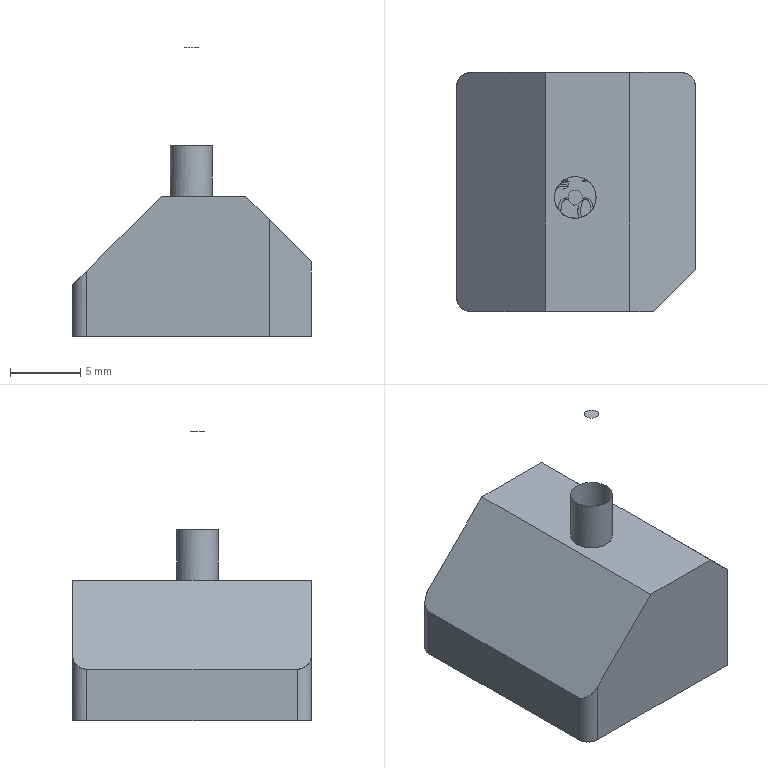NC program | PowerMill | posted with a generic post | part box 17 x 17 x 20.603 mm
Lines 37760 to 38492 of 42778:
N37857 M6
N37858 S18000 M03
N37859 G00 G90 X0.002 Y0.0
N37860 G43 Z9.803 H7
N37861
N37862 G05 P10000 R8
N37863 X9.8295 Y-5.6395
N37864 Z-14.7717
N37865 G01 Z-15.9717 F1200.0
N37866 X8.5944 Y-6.8746 Z-14.7367 F2000.0
N37867 X7.7228 Y-7.7462 Z-13.865
N37868 X7.4418 Y-8.0272 Z-13.5851
N37869 X7.1609 Y-8.3081 Z-13.3053
N37870 X6.8798 Y-8.5892 Z-13.0257
N37871 X6.7816 Y-8.6026 Z-12.9282
N37872 X7.0752 Y-8.309 Z-13.218
N37873 X7.8104 Y-7.5737 Z-13.9517
N37874 X8.6699 Y-6.7142 Z-14.8116
N37875 X9.8829 Y-5.5013 Z-16.025
N37876 X9.9345 Y-5.3648 Z-16.0781
N37877 X9.9048 Y-5.3945 Z-16.0479
N37878 X9.6356 Y-5.6637 Z-15.7768
N37879 X9.3656 Y-5.9337 Z-15.5072
N37880 X9.0957 Y-6.2036 Z-15.2376
N37881 X8.5216 Y-6.7777 Z-14.6631
N37882 X7.7273 Y-7.572 Z-13.8684
N37883 X7.3416 Y-7.9577 Z-13.4833
N37884 X6.9702 Y-8.3291 Z-13.112
N37885 X6.701 Y-8.5983 Z-12.8472
N37886 X6.6093 Y-8.6052 Z-12.756
N37887 X6.9039 Y-8.3106 Z-13.0467
N37888 X7.4978 Y-7.7166 Z-13.6392
N37889 X8.2992 Y-6.9152 Z-14.441
N37890 X9.0123 Y-6.2022 Z-15.1535
N37891 X9.3516 Y-5.8629 Z-15.4929
N37892 X9.6193 Y-5.5952 Z-15.7625
N37893 X9.9412 Y-5.2733 Z-16.0867
N37894 X9.9641 Y-5.2504 Z-16.1098
N37895 X9.9915 Y-5.1381 Z-16.1391
N37896 X9.872 Y-5.2576 Z-16.0174
N37897 X9.6054 Y-5.5242 Z-15.7477
N37898 X9.3296 Y-5.8 Z-15.4712
N37899 X8.9941 Y-6.1355 Z-15.1351
N37900 X8.2311 Y-6.8985 Z-14.3728
N37901 X7.4921 Y-7.6375 Z-13.6332
N37902 X7.1025 Y-8.0271 Z-13.2441
N37903 X6.782 Y-8.3476 Z-12.9248
N37904 X6.5202 Y-8.6094 Z-12.667
N37905 X6.4344 Y-8.6104 Z-12.5815
N37906 X6.6167 Y-8.428 Z-12.7612
N37907 X6.7988 Y-8.246 Z-12.9414
N37908 X6.9807 Y-8.0641 Z-13.1221
N37909 X7.3183 Y-7.7265 Z-13.4599
N37910 X7.9832 Y-7.0616 Z-14.1246
N37911 X8.8697 Y-6.1751 Z-15.0108
N37912 X9.2937 Y-5.751 Z-15.4354
N37913 X9.6371 Y-5.4076 Z-15.7792
N37914 X9.9348 Y-5.1099 Z-16.0802
N37915 X9.9922 Y-5.0526 Z-16.1388
N37916 X9.9871 Y-4.9728 Z-16.1343
N37917 X9.9382 Y-5.0217 Z-16.0844
N37918 X9.6271 Y-5.3328 Z-15.7697
N37919 X9.3152 Y-5.6447 Z-15.4566
N37920 X8.8493 Y-6.1106 Z-14.9908
N37921 X7.9104 Y-7.0495 Z-14.0519
N37922 X7.2311 Y-7.7288 Z-13.3727
N37923 X6.8845 Y-8.0754 Z-13.026
N37924 X6.7064 Y-8.2535 Z-12.8491
N37925 X6.528 Y-8.4319 Z-12.6726
N37926 X6.3494 Y-8.6105 Z-12.4966
N37927 X6.2647 Y-8.6104 Z-12.4118
N37928 X6.4471 Y-8.4279 Z-12.5916
N37929 X6.6293 Y-8.2457 Z-12.7719
N37930 X6.8113 Y-8.0638 Z-12.9527
N37931 X7.1489 Y-7.7261 Z-13.2905
N37932 X7.7898 Y-7.0853 Z-13.9313
N37933 X8.6032 Y-6.2719 Z-14.7447
N37934 X9.004 Y-5.871 Z-15.1458
N37935 X9.3524 Y-5.5226 Z-15.4932
N37936 X9.5245 Y-5.3505 Z-15.6664
N37937 X9.6998 Y-5.1753 Z-15.8414
N37938 X9.8121 Y-5.063 Z-15.9536
N37939 X9.9233 Y-4.9517 Z-16.0679
N37940 X9.99 Y-4.885 Z-16.1385
N37941 X9.9919 Y-4.7983 Z-16.14
N37942 X9.9538 Y-4.8364 Z-16.1002
N37943 X9.7637 Y-5.0264 Z-15.9057
N37944 X9.5786 Y-5.2116 Z-15.7204
N37945 X9.3976 Y-5.3926 Z-15.5384
N37946 X9.0342 Y-5.756 Z-15.176
N37947 X8.6872 Y-6.103 Z-14.8287
N37948 X7.7836 Y-7.0066 Z-13.9251
N37949 X7.0632 Y-7.727 Z-13.2047
N37950 X6.7256 Y-8.0646 Z-12.867
N37951 X6.5439 Y-8.2463 Z-12.6865
N37952 X6.362 Y-8.4282 Z-12.5065
N37953 X6.1798 Y-8.6104 Z-12.3269
N37954 X6.0952 Y-8.6102 Z-12.2422
N37955 X6.3856 Y-8.3198 Z-12.5274
N37956 X6.6923 Y-8.0131 Z-12.8339
N37957 X8.0252 Y-6.6801 Z-14.1669
N37958 X8.8562 Y-5.8491 Z-14.9975
N37959 X9.2693 Y-5.4361 Z-15.4107
N37960 X9.6218 Y-5.0835 Z-15.7651
N37961 X9.9887 Y-4.7167 Z-16.1348
N37962 X9.9892 Y-4.6313 Z-16.1372
N37963 X9.9529 Y-4.6676 Z-16.0995
N37964 X9.7279 Y-4.8926 Z-15.8699
N37965 X9.5332 Y-5.0873 Z-15.675
N37966 X9.3477 Y-5.2728 Z-15.4886
N37967 X8.9844 Y-5.636 Z-15.1262
N37968 X8.2034 Y-6.4171 Z-14.3449
N37969 X6.612 Y-8.0085 Z-12.7536
N37970 X6.301 Y-8.3195 Z-12.4428
N37971 X6.0103 Y-8.6102 Z-12.1574
N37972 X5.926 Y-8.6097 Z-12.0729
N37973 X6.1753 Y-8.3603 Z-12.3175
N37974 X6.4765 Y-8.0591 Z-12.618
N37975 X6.8365 Y-7.6992 Z-12.9776
N37976 X7.9813 Y-6.5543 Z-14.123
N37977 X9.0248 Y-5.5108 Z-15.1666
N37978 X9.3785 Y-5.1572 Z-15.5192
N37979 X9.5528 Y-4.9828 Z-15.6947
N37980 X9.7346 Y-4.801 Z-15.8763
N37981 X9.9279 Y-4.6078 Z-16.0735
N37982 X9.9912 Y-4.5444 Z-16.1396
N37983 X9.9887 Y-4.4621 Z-16.1347
N37984 X9.9322 Y-4.5186 Z-16.0758
N37985 X9.7519 Y-4.6989 Z-15.8928
N37986 X9.5703 Y-4.8805 Z-15.7122
N37987 X9.3175 Y-5.1333 Z-15.459
N37988 X8.8659 Y-5.5848 Z-15.0073
N37989 X7.9079 Y-6.5429 Z-14.0496
N37990 X7.0333 Y-7.4175 Z-13.1744
N37991 X6.5788 Y-7.872 Z-12.7203
N37992 X6.1968 Y-8.254 Z-12.3397
N37993 X5.8417 Y-8.609 Z-11.9883
N37994 X5.7579 Y-8.608 Z-11.9038
N37995 X6.1497 Y-8.2162 Z-12.2921
N37996 X6.5879 Y-7.778 Z-12.7296
N37997 X7.0988 Y-7.2671 Z-13.24
N37998 X8.1941 Y-6.1718 Z-14.3356
N37999 X8.8683 Y-5.4976 Z-15.0101
N38000 X9.3224 Y-5.0436 Z-15.4632
N38001 X9.5213 Y-4.8446 Z-15.663
N38002 X9.7209 Y-4.645 Z-15.8629
N38003 X9.9444 Y-4.4215 Z-16.0908
N38004 X9.9892 Y-4.3767 Z-16.1372
N38005 X9.9887 Y-4.2924 Z-16.1349
N38006 X9.5749 Y-4.7062 Z-15.718
N38007 X9.1731 Y-5.108 Z-15.3145
N38008 X8.6996 Y-5.5815 Z-14.8408
N38009 X7.7517 Y-6.5294 Z-13.8934
N38010 X6.7849 Y-7.4961 Z-12.9261
N38011 X6.3346 Y-7.9465 Z-12.476
N38012 X5.9716 Y-8.3095 Z-12.1148
N38013 X5.6691 Y-8.6119 Z-11.8163
N38014 X5.5848 Y-8.6115 Z-11.732
N38015 X5.8206 Y-8.3756 Z-11.9638
N38016 X6.2028 Y-7.9935 Z-12.3441
N38017 X6.6752 Y-7.521 Z-12.8164
N38018 X7.5586 Y-6.6377 Z-13.7002
N38019 X8.5855 Y-5.6107 Z-14.7271
N38020 X9.0424 Y-5.1538 Z-15.1839
N38021 X9.415 Y-4.7812 Z-15.5562
N38022 X9.6042 Y-4.592 Z-15.7456
N38023 X9.7278 Y-4.4684 Z-15.8694
N38024 X9.842 Y-4.3542 Z-15.9843
N38025 X9.9897 Y-4.2065 Z-16.1381
N38026 X9.9887 Y-4.1227 Z-16.1344
N38027 X9.9157 Y-4.1957 Z-16.0594
N38028 X9.7916 Y-4.3198 Z-15.9337
N38029 X9.6672 Y-4.4442 Z-15.8086
N38030 X9.5427 Y-4.5687 Z-15.6838
N38031 X9.4181 Y-4.6933 Z-15.5591
N38032 X9.2842 Y-4.8272 Z-15.4254
N38033 X9.1595 Y-4.9519 Z-15.301
N38034 X9.0348 Y-5.0766 Z-15.1765
N38035 X8.9101 Y-5.2013 Z-15.0521
N38036 X8.7855 Y-5.3259 Z-14.9273
N38037 X7.6722 Y-6.4391 Z-13.8139
N38038 X6.1063 Y-8.0051 Z-12.248
N38039 X5.9059 Y-8.2055 Z-12.0478
N38040 X5.705 Y-8.4064 Z-11.8487
N38041 X5.5036 Y-8.6077 Z-11.6504
N38042 X5.4174 Y-8.6091 Z-11.5638
N38043 X5.8117 Y-8.2148 Z-11.9543
N38044 X6.2455 Y-7.781 Z-12.3871
N38045 X6.7615 Y-7.2651 Z-12.9026
N38046 X7.959 Y-6.0676 Z-14.1005
N38047 X8.7835 Y-5.243 Z-14.9253
N38048 X9.2225 Y-4.804 Z-15.3633
N38049 X9.4556 Y-4.5709 Z-15.5975
N38050 X9.702 Y-4.3246 Z-15.8434
N38051 X9.8192 Y-4.2074 Z-15.9606
N38052 X9.9275 Y-4.099 Z-16.0728
N38053 X9.9906 Y-4.0359 Z-16.1391
N38054 X9.989 Y-3.9526 Z-16.1368
N38055 X9.9791 Y-3.9625 Z-16.1265
N38056 X9.7443 Y-4.1974 Z-15.8865
N38057 X9.4805 Y-4.4612 Z-15.6222
N38058 X9.2183 Y-4.7233 Z-15.3593
N38059 X8.7471 Y-5.1945 Z-14.8889
N38060 X7.8687 Y-6.0729 Z-14.0103
N38061 X6.6113 Y-7.3303 Z-12.7531
N38062 X6.3603 Y-7.5813 Z-12.5026
N38063 X6.1096 Y-7.832 Z-12.2513
N38064 X5.859 Y-8.0826 Z-12.0
N38065 X5.608 Y-8.3336 Z-11.7495
N38066 X5.3559 Y-8.5857 Z-11.5011
N38067 X5.3054 Y-8.5515 Z-11.4491
N38068 X5.6985 Y-8.1583 Z-11.8397
N38069 X6.0906 Y-7.7662 Z-12.2324
N38070 X6.4829 Y-7.3739 Z-12.6247
N38071 X8.055 Y-5.8018 Z-14.1965
N38072 X8.8228 Y-5.034 Z-14.9645
N38073 X9.3339 Y-4.5229 Z-15.4751
N38074 X9.6143 Y-4.2425 Z-15.7556
N38075 X9.8716 Y-3.9852 Z-16.0149
N38076 X9.9936 Y-3.8632 Z-16.1407
N38077 X9.9887 Y-3.7832 Z-16.1356
N38078 X9.8269 Y-3.945 Z-15.9701
N38079 X9.5333 Y-4.2387 Z-15.6747
N38080 X9.2369 Y-4.5351 Z-15.3781
N38081 X8.7308 Y-5.0412 Z-14.8724
N38082 X7.0545 Y-6.7174 Z-13.1961
N38083 X6.1659 Y-7.606 Z-12.3076
N38084 X5.2773 Y-8.4947 Z-11.4193
N38085 X5.2524 Y-8.4347 Z-11.3944
N38086 X6.2201 Y-7.467 Z-12.3617
N38087 X7.1877 Y-6.4994 Z-13.3292
N38088 X8.8209 Y-4.8662 Z-14.9626
N38089 X9.3274 Y-4.3597 Z-15.4686
N38090 X9.604 Y-4.0831 Z-15.7453
N38091 X9.8626 Y-3.8245 Z-16.0057
N38092 X9.9934 Y-3.6937 Z-16.1407
N38093 X9.993 Y-3.6092 Z-16.1405
N38094 X9.8247 Y-3.7775 Z-15.9673
N38095 X9.5715 Y-4.0307 Z-15.713
N38096 X9.3059 Y-4.2963 Z-15.4471
N38097 X8.8165 Y-4.7858 Z-14.9582
N38098 X7.7755 Y-5.8267 Z-13.9171
N38099 X5.2292 Y-8.373 Z-11.3711
N38100 X5.2132 Y-8.3042 Z-11.3565
N38101 X5.7159 Y-7.8015 Z-11.8572
N38102 X6.2178 Y-7.2996 Z-12.3597
N38103 X6.7199 Y-6.7975 Z-12.8615
N38104 X8.6247 Y-4.8927 Z-14.7663
N38105 X9.0659 Y-4.4515 Z-15.2069
N38106 X9.3564 Y-4.161 Z-15.4979
N38107 X9.5897 Y-3.9277 Z-15.7311
N38108 X9.7042 Y-3.8132 Z-15.8458
N38109 X9.8159 Y-3.7015 Z-15.9574
N38110 X9.9262 Y-3.5912 Z-16.0716
N38111 X9.9903 Y-3.5271 Z-16.1388
N38112 X9.9935 Y-3.439 Z-16.1407
N38113 X9.8707 Y-3.5618 Z-16.014
N38114 X9.6131 Y-3.8195 Z-15.7544
N38115 X9.3334 Y-4.0992 Z-15.4746
N38116 X8.8223 Y-4.6103 Z-14.964
N38117 X6.5344 Y-6.8981 Z-12.676
N38118 X5.8782 Y-7.5543 Z-12.0197
N38119 X5.6527 Y-7.7798 Z-11.7953
N38120 X5.4272 Y-8.0053 Z-11.571
N38121 X5.2016 Y-8.2309 Z-11.3467
N38122 X5.191 Y-8.1566 Z-11.3369
N38123 X5.6119 Y-7.7358 Z-11.7549
N38124 X6.0507 Y-7.297 Z-12.1921
N38125 X6.8099 Y-6.5378 Z-12.9515
N38126 X8.8051 Y-4.5426 Z-14.9468
N38127 X9.2669 Y-4.0807 Z-15.4079
N38128 X9.5147 Y-3.833 Z-15.6564
N38129 X9.7327 Y-3.615 Z-15.8743
N38130 X9.9248 Y-3.4229 Z-16.07
N38131 X9.9921 Y-3.3556 Z-16.1401
N38132 X9.9933 Y-3.2696 Z-16.1406
N38133 X9.8531 Y-3.4097 Z-15.9961
N38134 X9.5963 Y-3.6666 Z-15.7376
N38135 X9.3225 Y-3.9403 Z-15.4637
N38136 X8.8194 Y-4.4434 Z-14.9611
N38137 X7.632 Y-5.6309 Z-13.7736
N38138 X5.462 Y-7.8009 Z-11.6039
N38139 X5.1804 Y-8.0824 Z-11.3269
N38140 X5.1699 Y-8.0081 Z-11.3169
N38141 X5.4025 Y-7.7755 Z-11.5472
N38142 X5.6354 Y-7.5426 Z-11.777
N38143 X6.0886 Y-7.0893 Z-12.23
N38144 X6.7321 Y-6.4459 Z-12.8737
N38145 X8.7806 Y-4.3974 Z-14.9223
N38146 X9.2374 Y-3.9405 Z-15.3783
N38147 X9.4766 Y-3.7014 Z-15.6185
N38148 X9.7202 Y-3.4578 Z-15.8617
N38149 X9.9338 Y-3.2442 Z-16.0796
N38150 X9.9915 Y-3.1865 Z-16.1398
N38151 X9.9889 Y-3.1043 Z-16.1363
N38152 X9.9154 Y-3.1777 Z-16.0606
N38153 X9.6677 Y-3.4255 Z-15.8092
N38154 X9.403 Y-3.6902 Z-15.5448
N38155 X9.128 Y-3.9651 Z-15.269
N38156 X8.5778 Y-4.5153 Z-14.7194
N38157 X7.3147 Y-5.7785 Z-13.4563
N38158 X6.3051 Y-6.788 Z-12.4467
N38159 X5.8452 Y-7.2479 Z-11.9867
N38160 X5.5943 Y-7.4988 Z-11.7363
N38161 X5.3478 Y-7.7453 Z-11.489
N38162 X5.1684 Y-7.9247 Z-11.3144
N38163 X5.1657 Y-7.8426 Z-11.3129
N38164 X5.3479 Y-7.6604 Z-11.4899
N38165 X5.5086 Y-7.4997 Z-11.6498
N38166 X5.762 Y-7.2462 Z-11.9033
N38167 X6.2445 Y-6.7637 Z-12.3862
N38168 X6.797 Y-6.2113 Z-12.9385
N38169 X8.7527 Y-4.2556 Z-14.8943
N38170 X9.3187 Y-3.6896 Z-15.4602
N38171 X9.501 Y-3.5073 Z-15.643
N38172 X9.6838 Y-3.3245 Z-15.8248
N38173 X9.8892 Y-3.1191 Z-16.0319
N38174 X9.994 Y-3.0143 Z-16.1409
N38175 X9.992 Y-2.9314 Z-16.1401
N38176 X9.9163 Y-3.0071 Z-16.0613
N38177 X9.6957 Y-3.2277 Z-15.837
N38178 X9.4218 Y-3.5016 Z-15.5636
N38179 X9.1756 Y-3.7479 Z-15.3164
N38180 X8.6842 Y-4.2392 Z-14.8259
N38181 X6.5313 Y-6.3921 Z-12.6729
N38182 X6.0445 Y-6.8789 Z-12.1858
N38183 X5.6733 Y-7.2501 Z-11.8149
N38184 X5.455 Y-7.4684 Z-11.5962
N38185 X5.3174 Y-7.606 Z-11.46
N38186 X5.1636 Y-7.7598 Z-11.3116
N38187 X5.163 Y-7.6756 Z-11.3112
N38188 X5.3218 Y-7.5168 Z-11.4635
N38189 X5.4854 Y-7.3532 Z-11.6269
N38190 X6.1217 Y-6.7169 Z-12.2634
N38191 X6.9601 Y-5.8785 Z-13.1016
N38192 X8.6697 Y-4.1689 Z-14.8112
N38193 X9.281 Y-3.5576 Z-15.4224
N38194 X9.4643 Y-3.3743 Z-15.6063
N38195 X9.6481 Y-3.1905 Z-15.7892
N38196 X9.8366 Y-3.002 Z-15.9782
N38197 X9.9942 Y-2.8444 Z-16.1409
N38198 X9.9934 Y-2.7603 Z-16.1407
N38199 X9.8678 Y-2.886 Z-16.011
N38200 X9.6087 Y-3.145 Z-15.75
N38201 X9.3308 Y-3.423 Z-15.472
N38202 X8.8212 Y-3.9325 Z-14.9629
N38203 X7.5458 Y-5.2079 Z-13.6874
N38204 X5.6115 Y-7.1422 Z-11.7529
N38205 X5.4486 Y-7.3051 Z-11.5901
N38206 X5.3277 Y-7.426 Z-11.4696
N38207 X5.1626 Y-7.5912 Z-11.3109
N38208 X5.1622 Y-7.5067 Z-11.3105
N38209 X5.2896 Y-7.3792 Z-11.432
N38210 X5.4815 Y-7.1874 Z-11.6228
N38211 X5.7014 Y-6.9674 Z-11.8428
N38212 X6.0602 Y-6.6087 Z-12.2015
N38213 X6.5186 Y-6.1502 Z-12.6602
N38214 X8.8137 Y-3.8552 Z-14.9554
N38215 X9.2939 Y-3.375 Z-15.4349
N38216 X9.5531 Y-3.1158 Z-15.6946
N38217 X9.8032 Y-2.8656 Z-15.9455
N38218 X9.9928 Y-2.6761 Z-16.1405
N38219 X9.9932 Y-2.5908 Z-16.1406
N38220 X9.8448 Y-2.7393 Z-15.9876
N38221 X9.589 Y-2.995 Z-15.7304
N38222 X9.3175 Y-3.2665 Z-15.4587
N38223 X8.8186 Y-3.7654 Z-14.9603
N38224 X6.8707 Y-5.7133 Z-13.0122
N38225 X6.0763 Y-6.5077 Z-12.2181
N38226 X5.4657 Y-7.1183 Z-11.6073
N38227 X5.3119 Y-7.2721 Z-11.4537
N38228 X5.1624 Y-7.4216 Z-11.3107
N38229 X5.162 Y-7.3371 Z-11.3103
N38230 X5.3055 Y-7.1937 Z-11.4473
N38231 X5.4527 Y-7.0465 Z-11.5942
N38232 X6.0688 Y-6.4304 Z-12.2105
N38233 X6.8708 Y-5.6283 Z-13.0123
N38234 X8.811 Y-3.6882 Z-14.9527
N38235 X9.2843 Y-3.2149 Z-15.4253
N38236 X9.5399 Y-2.9592 Z-15.6816
N38237 X9.7386 Y-2.7605 Z-15.8802
N38238 X9.9299 Y-2.5693 Z-16.0751
N38239 X9.9926 Y-2.5066 Z-16.1404
N38240 X9.9918 Y-2.4225 Z-16.14
N38241 X9.9319 Y-2.4824 Z-16.0775
N38242 X9.7184 Y-2.6959 Z-15.8599
N38243 X9.4681 Y-2.9462 Z-15.61
N38244 X9.2249 Y-3.1894 Z-15.3658
N38245 X8.7429 Y-3.6714 Z-14.8846
N38246 X6.6334 Y-5.7809 Z-12.775
N38247 X6.0536 Y-6.3607 Z-12.195
N38248 X5.5913 Y-6.823 Z-11.7327
N38249 X5.4097 Y-7.0046 Z-11.5509
N38250 X5.2932 Y-7.1211 Z-11.4356
N38251 X5.1617 Y-7.2526 Z-11.3099
N38252 X5.1615 Y-7.168 Z-11.3096
N38253 X5.39 Y-6.9395 Z-11.5325
N38254 X5.7019 Y-6.6276 Z-11.8433
N38255 X6.5772 Y-5.7522 Z-12.7188
N38256 X8.619 Y-3.7105 Z-14.7606
N38257 X9.0866 Y-3.2428 Z-15.2276
N38258 X9.3753 Y-2.9542 Z-15.5168
N38259 X9.6143 Y-2.7152 Z-15.7556
N38260 X9.8542 Y-2.4752 Z-15.9977
N38261 X9.9914 Y-2.3381 Z-16.1397
N38262 X9.9913 Y-2.2533 Z-16.1396
N38263 X9.8513 Y-2.3933 Z-15.9947
N38264 X9.6117 Y-2.6329 Z-15.753
N38265 X9.3736 Y-2.871 Z-15.5152
N38266 X9.0706 Y-3.174 Z-15.2116
N38267 X8.6061 Y-3.6385 Z-14.7478
N38268 X6.5787 Y-5.666 Z-12.7202
N38269 X5.7004 Y-6.5442 Z-11.8419
N38270 X5.3896 Y-6.8551 Z-11.5321
N38271 X5.1615 Y-7.0831 Z-11.3096
N38272 X5.1614 Y-6.9983 Z-11.3095
N38273 X5.3891 Y-6.7706 Z-11.5317
N38274 X5.6989 Y-6.4609 Z-11.8403
N38275 X6.5803 Y-5.5794 Z-12.7219
N38276 X8.5904 Y-3.5694 Z-14.732
N38277 X9.0516 Y-3.1081 Z-15.1927
N38278 X9.372 Y-2.7877 Z-15.5136
N38279 X9.6091 Y-2.5506 Z-15.7505
N38280 X9.8484 Y-2.3114 Z-15.9918
N38281 X9.9912 Y-2.1686 Z-16.1396
N38282 Y-2.0837
N38283 X9.8478 Y-2.2271 Z-15.9912
N38284 X9.6086 Y-2.4663 Z-15.7499
N38285 X9.3717 Y-2.7032 Z-15.5133
N38286 X9.0497 Y-3.0252 Z-15.1908
N38287 X8.589 Y-3.4859 Z-14.7306
N38288 X6.581 Y-5.494 Z-12.7225
N38289 X5.6986 Y-6.3763 Z-11.84
N38290 X5.3891 Y-6.6858 Z-11.5316
N38291 X5.1614 Y-6.9135 Z-11.3095
N38292 Y-6.8286
N38293 X5.3891 Y-6.601 Z-11.5316
N38294 X5.6986 Y-6.2915 Z-11.84
N38295 X6.581 Y-5.4091 Z-12.7225
N38296 X8.5888 Y-3.4012 Z-14.7304
N38297 X9.0494 Y-2.9406 Z-15.1905
N38298 X9.3717 Y-2.6184 Z-15.5133
N38299 X9.6086 Y-2.3815 Z-15.7499
N38300 X9.8477 Y-2.1423 Z-15.9912
N38301 X9.9912 Y-1.9989 Z-16.1396
N38302 Y-1.914
N38303 X9.8478 Y-2.0574 Z-15.9912
N38304 X9.6086 Y-2.2966 Z-15.7499
N38305 X9.3717 Y-2.5335 Z-15.5133
N38306 X9.0503 Y-2.8549 Z-15.1914
N38307 X8.5897 Y-3.3155 Z-14.7313
N38308 X6.581 Y-5.3242 Z-12.7226
N38309 X5.6986 Y-6.2066 Z-11.84
N38310 X5.3891 Y-6.5161 Z-11.5316
N38311 X5.1614 Y-6.7438 Z-11.3095
N38312 Y-6.6589
N38313 X5.3891 Y-6.4313 Z-11.5316
N38314 X5.6986 Y-6.1217 Z-11.84
N38315 X6.5811 Y-5.2393 Z-12.7226
N38316 X8.5891 Y-3.2313 Z-14.7307
N38317 X9.0497 Y-2.7707 Z-15.1908
N38318 X9.3717 Y-2.4487 Z-15.5133
N38319 X9.6086 Y-2.2118 Z-15.7499
N38320 X9.8477 Y-1.9726 Z-15.9912
N38321 X9.9912 Y-1.8292 Z-16.1396
N38322 Y-1.7443
N38323 X9.8478 Y-1.8877 Z-15.9912
N38324 X9.6086 Y-2.1269 Z-15.7499
N38325 X9.3717 Y-2.3638 Z-15.5133
N38326 X9.051 Y-2.6845 Z-15.1921
N38327 X8.5903 Y-3.1452 Z-14.7319
N38328 X6.5813 Y-5.1542 Z-12.7228
N38329 X5.6985 Y-6.037 Z-11.84
N38330 X5.3891 Y-6.3464 Z-11.5316
N38331 X5.1614 Y-6.5741 Z-11.3095
N38332 Y-6.4892
N38333 X5.3891 Y-6.2616 Z-11.5316
N38334 X5.6986 Y-5.952 Z-11.84
N38335 X6.581 Y-5.0696 Z-12.7226
N38336 X8.5902 Y-3.0604 Z-14.7318
N38337 X9.0509 Y-2.5997 Z-15.192
N38338 X9.3717 Y-2.279 Z-15.5133
N38339 X9.6086 Y-2.042 Z-15.7499
N38340 X9.8478 Y-1.8028 Z-15.9912
N38341 X9.9912 Y-1.6595 Z-16.1396
N38342 Y-1.5746
N38343 X9.8478 Y-1.718 Z-15.9912
N38344 X9.6086 Y-1.9572 Z-15.7499
N38345 X9.3717 Y-2.1941 Z-15.5133
N38346 X9.0502 Y-2.5155 Z-15.1913
N38347 X8.5897 Y-2.9761 Z-14.7313
N38348 X6.5811 Y-4.9846 Z-12.7227
N38349 X5.6985 Y-5.8673 Z-11.8399
N38350 X5.3891 Y-6.1767 Z-11.5316
N38351 X5.1614 Y-6.4044 Z-11.3095
N38352 Y-6.3195
N38353 X5.3891 Y-6.0919 Z-11.5316
N38354 X5.6985 Y-5.7824 Z-11.8399
N38355 X6.581 Y-4.8999 Z-12.7225
N38356 X8.5901 Y-2.8909 Z-14.7317
N38357 X9.0507 Y-2.4302 Z-15.1918
N38358 X9.3717 Y-2.1093 Z-15.5133
N38359 X9.6086 Y-1.8724 Z-15.7499
N38360 X9.8478 Y-1.6332 Z-15.9912
N38361 X9.9912 Y-1.4898 Z-16.1396
N38362 Y-1.4049
N38363 X9.8478 Y-1.5483 Z-15.9912
N38364 X9.6086 Y-1.7875 Z-15.7499
N38365 X9.3717 Y-2.0244 Z-15.5133
N38366 X9.0509 Y-2.3451 Z-15.192
N38367 X8.5903 Y-2.8058 Z-14.7319
N38368 X6.5812 Y-4.8148 Z-12.7228
N38369 X5.6985 Y-5.6976 Z-11.8399
N38370 X5.3891 Y-6.007 Z-11.5316
N38371 X5.1614 Y-6.2347 Z-11.3095
N38372 Y-6.1498
N38373 X5.3891 Y-5.9221 Z-11.5316
N38374 X5.6986 Y-5.6126 Z-11.84
N38375 X6.5811 Y-4.7302 Z-12.7226
N38376 X8.5899 Y-2.7213 Z-14.7315
N38377 X9.0506 Y-2.2607 Z-15.1917
N38378 X9.3717 Y-1.9395 Z-15.5133
N38379 X9.6086 Y-1.7026 Z-15.7499
N38380 X9.8478 Y-1.4634 Z-15.9912
N38381 X9.9912 Y-1.3201 Z-16.1396
N38382 Y-1.2352
N38383 X9.8478 Y-1.3786 Z-15.9912
N38384 X9.6086 Y-1.6178 Z-15.7499
N38385 X9.3717 Y-1.8547 Z-15.5133
N38386 X9.0517 Y-2.1747 Z-15.1928
N38387 X8.591 Y-2.6354 Z-14.7326
N38388 X6.5811 Y-4.6453 Z-12.7227
N38389 X5.6986 Y-5.5278 Z-11.84
N38390 X5.3891 Y-5.8373 Z-11.5316
N38391 X5.1614 Y-6.065 Z-11.3095
N38392 Y-5.9801
N38393 X5.3891 Y-5.7524 Z-11.5316
N38394 X5.6986 Y-5.4429 Z-11.84
N38395 X6.5812 Y-4.5603 Z-12.7228
N38396 X8.5893 Y-2.5522 Z-14.7309
N38397 X9.0499 Y-2.0916 Z-15.191
N38398 X9.3717 Y-1.7698 Z-15.5133
N38399 X9.6086 Y-1.5329 Z-15.7499
N38400 X9.8478 Y-1.2937 Z-15.9912
N38401 X9.9912 Y-1.1503 Z-16.1396
N38402 Y-1.0655
N38403 X9.8478 Y-1.2088 Z-15.9913
N38404 X9.6086 Y-1.4481 Z-15.7499
N38405 X9.3717 Y-1.685 Z-15.5133
N38406 X9.0496 Y-2.0071 Z-15.1907
N38407 X8.5889 Y-2.4678 Z-14.7305
N38408 X6.5811 Y-4.4755 Z-12.7227
N38409 X5.6986 Y-5.3581 Z-11.84
N38410 X5.3891 Y-5.6676 Z-11.5316
N38411 X5.1614 Y-5.8953 Z-11.3095
N38412 Y-5.8104
N38413 X5.3891 Y-5.5827 Z-11.5316
N38414 X5.6986 Y-5.2732 Z-11.84
N38415 X6.5811 Y-4.3907 Z-12.7227
N38416 X8.5887 Y-2.3831 Z-14.7303
N38417 X9.0493 Y-1.9225 Z-15.1904
N38418 X9.3717 Y-1.6001 Z-15.5133
N38419 X9.6085 Y-1.3633 Z-15.7499
N38420 X9.8477 Y-1.1241 Z-15.9911
N38421 X9.9912 Y-0.9806 Z-16.1396
N38422 Y-0.8958
N38423 X9.8478 Y-1.0392 Z-15.9912
N38424 X9.6086 Y-1.2784 Z-15.7499
N38425 X9.3717 Y-1.5153 Z-15.5133
N38426 X9.0498 Y-1.8371 Z-15.1909
N38427 X8.5891 Y-2.2978 Z-14.7307
N38428 X6.5811 Y-4.3059 Z-12.7226
N38429 X5.6986 Y-5.1884 Z-11.84
N38430 X5.3891 Y-5.4979 Z-11.5316
N38431 X5.1614 Y-5.7256 Z-11.3095
N38432 Y-5.6407
N38433 X5.3891 Y-5.413 Z-11.5316
N38434 X5.6986 Y-5.1035 Z-11.84
N38435 X6.581 Y-4.2211 Z-12.7226
N38436 X8.589 Y-2.2131 Z-14.7306
N38437 X9.0496 Y-1.7525 Z-15.1907
N38438 X9.3717 Y-1.4304 Z-15.5133
N38439 X9.6086 Y-1.1936 Z-15.7499
N38440 X9.8477 Y-0.9544 Z-15.9912
N38441 X9.9912 Y-0.8109 Z-16.1396
N38442 Y-0.7261
N38443 X9.8477 Y-0.8695 Z-15.9911
N38444 X9.6085 Y-1.1087 Z-15.7499
N38445 X9.3717 Y-1.3456 Z-15.5133
N38446 X9.0504 Y-1.6668 Z-15.1915
N38447 X8.5899 Y-2.1274 Z-14.7315
N38448 X6.5813 Y-4.136 Z-12.7228
N38449 X5.6986 Y-5.0187 Z-11.84
N38450 X5.3891 Y-5.3282 Z-11.5316
N38451 X5.1614 Y-5.5559 Z-11.3095
N38452 Y-5.471
N38453 X5.3891 Y-5.2433 Z-11.5316
N38454 X5.6986 Y-4.9338 Z-11.84
N38455 X6.5811 Y-4.0513 Z-12.7226
N38456 X8.5905 Y-2.0419 Z-14.7321
N38457 X9.0512 Y-1.5812 Z-15.1923
N38458 X9.3717 Y-1.2607 Z-15.5133
N38459 X9.6085 Y-1.0239 Z-15.7499
N38460 X9.8477 Y-0.7847 Z-15.9911
N38461 X9.9912 Y-0.6412 Z-16.1396
N38462 Y-0.5564
N38463 X9.8477 Y-0.6998 Z-15.9912
N38464 X9.6085 Y-0.939 Z-15.7499
N38465 X9.3717 Y-1.1759 Z-15.5133
N38466 X9.0517 Y-1.4958 Z-15.1928
N38467 X8.5911 Y-1.9564 Z-14.7327
N38468 X6.5813 Y-3.9663 Z-12.7228
N38469 X5.6986 Y-4.849 Z-11.84
N38470 X5.3891 Y-5.1585 Z-11.5316
N38471 X5.1614 Y-5.3861 Z-11.3095
N38472 Y-5.3013
N38473 X5.3891 Y-5.0736 Z-11.5316
N38474 X5.6986 Y-4.7641 Z-11.84
N38475 X6.581 Y-3.8817 Z-12.7226
N38476 X8.5887 Y-1.8739 Z-14.7304
N38477 X9.0493 Y-1.4134 Z-15.1904
N38478 X9.3717 Y-1.091 Z-15.5133
N38479 X9.6086 Y-0.8541 Z-15.7499
N38480 X9.8478 Y-0.6149 Z-15.9912
N38481 X9.9912 Y-0.4715 Z-16.1396
N38482 Y-0.3867
N38483 X9.8477 Y-0.5301 Z-15.9912
N38484 X9.6086 Y-0.7693 Z-15.7499
N38485 X9.3717 Y-1.0062 Z-15.5133
N38486 X9.0508 Y-1.327 Z-15.1919
N38487 X8.5901 Y-1.7877 Z-14.7317
N38488 X6.581 Y-3.7968 Z-12.7226
N38489 X5.6986 Y-4.6792 Z-11.84
N38490 X5.3891 Y-4.9888 Z-11.5316
N38491 X5.1614 Y-5.2164 Z-11.3095
N38492 Y-5.1316
N38493 X5.3891 Y-4.9039 Z-11.5316
N38494 X5.6986 Y-4.5944 Z-11.84
N38495 X6.5814 Y-3.7116 Z-12.7229
N38496 X8.5881 Y-1.7049 Z-14.7297
N38497 X9.0487 Y-1.2443 Z-15.1898
N38498 X9.3717 Y-0.9213 Z-15.5133
N38499 X9.6086 Y-0.6844 Z-15.7499
N38500 X9.8478 Y-0.4452 Z-15.9912
N38501 X9.9912 Y-0.3018 Z-16.1396
N38502 Y-0.217
N38503 X9.8477 Y-0.3604 Z-15.9911
N38504 X9.6085 Y-0.5996 Z-15.7499
N38505 X9.3717 Y-0.8365 Z-15.5133
N38506 X9.0508 Y-1.1573 Z-15.1919
N38507 X8.5902 Y-1.6179 Z-14.7318
N38508 X6.5811 Y-3.627 Z-12.7227
N38509 X5.6986 Y-4.5095 Z-11.8401
N38510 X5.3891 Y-4.8191 Z-11.5316
N38511 X5.1614 Y-5.0467 Z-11.3095
N38512 Y-4.9619
N38513 X5.3891 Y-4.7342 Z-11.5316
N38514 X5.6986 Y-4.4247 Z-11.84
N38515 X6.5814 Y-3.5419 Z-12.7229
N38516 X8.5937 Y-1.5296 Z-14.7353
N38517 X9.0544 Y-1.0688 Z-15.1955
N38518 X9.3717 Y-0.7516 Z-15.5133
N38519 X9.6085 Y-0.5148 Z-15.7499
N38520 X9.8477 Y-0.2756 Z-15.9911
N38521 X9.9912 Y-0.1321 Z-16.1396
N38522 Y-0.0473
N38523 X9.8477 Y-0.1907 Z-15.9911
N38524 X9.6086 Y-0.4299 Z-15.7499
N38525 X9.3717 Y-0.6668 Z-15.5133
N38526 X9.0516 Y-0.9868 Z-15.1927
N38527 X8.5909 Y-1.4475 Z-14.7326
N38528 X6.5811 Y-3.4573 Z-12.7227
N38529 X5.6985 Y-4.3399 Z-11.8399
N38530 X5.3891 Y-4.6494 Z-11.5316
N38531 X5.1614 Y-4.877 Z-11.3095
N38532 Y-4.7922
N38533 X5.3891 Y-4.5645 Z-11.5316
N38534 X5.6985 Y-4.2551 Z-11.8399
N38535 X6.5811 Y-3.3725 Z-12.7227
N38536 X8.5907 Y-1.3628 Z-14.7323
N38537 X9.0515 Y-0.9021 Z-15.1926
N38538 X9.3717 Y-0.5819 Z-15.5133
N38539 X9.6086 Y-0.345 Z-15.7499
N38540 X9.8477 Y-0.1058 Z-15.9912
N38541 X9.9912 Y0.0376 Z-16.1396
N38542 Y0.1224
N38543 X9.8478 Y-0.021 Z-15.9912
N38544 X9.6086 Y-0.2602 Z-15.7499
N38545 X9.3717 Y-0.497 Z-15.5133
N38546 X9.05 Y-0.8188 Z-15.1911
N38547 X8.5893 Y-1.2794 Z-14.7309
N38548 X6.581 Y-3.2877 Z-12.7226
N38549 X5.6985 Y-4.1702 Z-11.8399
N38550 X5.3891 Y-4.4797 Z-11.5316
N38551 X5.1614 Y-4.7073 Z-11.3095
N38552 Y-4.6225
N38553 X5.3891 Y-4.3948 Z-11.5316
N38554 X5.6985 Y-4.0854 Z-11.8399
N38555 X6.5812 Y-3.2026 Z-12.7228
N38556 X8.5897 Y-1.1941 Z-14.7313
N38557 X9.0503 Y-0.7336 Z-15.1914
N38558 X9.3717 Y-0.4122 Z-15.5133
N38559 X9.6086 Y-0.1753 Z-15.7499
N38560 X9.8477 Y0.0639 Z-15.9912
N38561 X9.9912 Y0.2073 Z-16.1396
N38562 Y0.2922
N38563 X9.8477 Y0.1487 Z-15.9912
N38564 X9.6086 Y-0.0905 Z-15.7499
N38565 X9.3717 Y-0.3273 Z-15.5133
N38566 X9.0506 Y-0.6485 Z-15.1917
N38567 X8.59 Y-1.1091 Z-14.7316
N38568 X6.5811 Y-3.118 Z-12.7226
N38569 X5.6985 Y-4.0005 Z-11.84
N38570 X5.3891 Y-4.3099 Z-11.5316
N38571 X5.1614 Y-4.5376 Z-11.3095
N38572 Y-4.4528
N38573 X5.3891 Y-4.2251 Z-11.5316
N38574 X5.6986 Y-3.9156 Z-11.84
N38575 X6.5809 Y-3.0333 Z-12.7225
N38576 X8.5889 Y-1.0253 Z-14.7305
N38577 X9.0494 Y-0.5647 Z-15.1905
N38578 X9.3717 Y-0.2425 Z-15.5133
N38579 X9.6086 Y-0.0056 Z-15.7499
N38580 X9.8478 Y0.2336 Z-15.9912
N38581 X9.9912 Y0.377 Z-16.1396
N38582 Y0.4619
N38583 X9.8477 Y0.3184 Z-15.9912
N38584 X9.6086 Y0.0792 Z-15.7499
N38585 X9.3717 Y-0.1576 Z-15.5133
N38586 X9.0493 Y-0.48 Z-15.1904
N38587 X8.5887 Y-0.9406 Z-14.7304
N38588 X6.581 Y-2.9483 Z-12.7226
N38589 X5.6985 Y-3.8308 Z-11.84